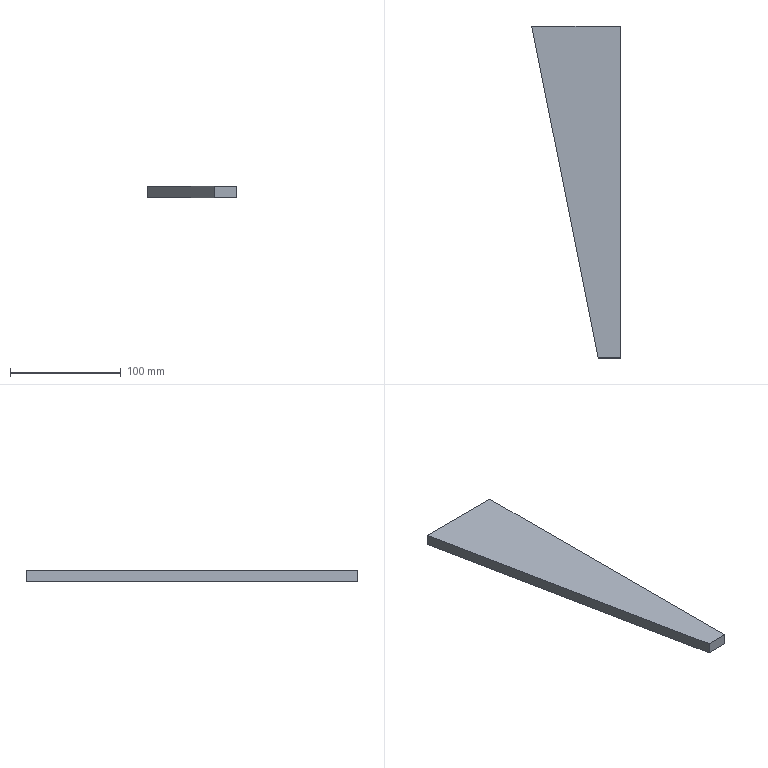Part | SolidWorks | features Extrusion 1 | 1 solid | 6 faces | box 80 x 300 x 10 mm | volume 150000 mm3 | plane 6
STEP:
#1=CARTESIAN_POINT('',(-80.,0.,-5.));
#2=VERTEX_POINT('',#1);
#3=CARTESIAN_POINT('',(-20.,-300.,-5.));
#4=VERTEX_POINT('',#3);
#5=CARTESIAN_POINT('',(-20.,-300.,-5.));
#6=DIRECTION('',(0.1961,-0.9806,0.));
#7=VECTOR('',#6,1000.);
#8=LINE('',#5,#7);
#9=EDGE_CURVE('',#2,#4,#8,.T.);
#10=ORIENTED_EDGE('',*,*,#9,.T.);
#11=CARTESIAN_POINT('',(-20.,-300.,5.));
#12=VERTEX_POINT('',#11);
#13=CARTESIAN_POINT('',(-20.,-300.,5.));
#14=DIRECTION('',(0.,0.,-1.));
#15=VECTOR('',#14,1000.);
#16=LINE('',#13,#15);
#17=EDGE_CURVE('',#12,#4,#16,.T.);
#18=ORIENTED_EDGE('',*,*,#17,.F.);
#19=CARTESIAN_POINT('',(-80.,0.,5.));
#20=VERTEX_POINT('',#19);
#21=CARTESIAN_POINT('',(-20.,-300.,5.));
#22=DIRECTION('',(0.1961,-0.9806,0.));
#23=VECTOR('',#22,1000.);
#24=LINE('',#21,#23);
#25=EDGE_CURVE('',#20,#12,#24,.T.);
#26=ORIENTED_EDGE('',*,*,#25,.F.);
#27=CARTESIAN_POINT('',(-80.,0.,5.));
#28=DIRECTION('',(0.,0.,-1.));
#29=VECTOR('',#28,1000.);
#30=LINE('',#27,#29);
#31=EDGE_CURVE('',#20,#2,#30,.T.);
#32=ORIENTED_EDGE('',*,*,#31,.T.);
#33=EDGE_LOOP('',(#10,#18,#26,#32));
#34=FACE_OUTER_BOUND('',#33,.T.);
#35=CARTESIAN_POINT('',(-20.,-300.,5.));
#36=DIRECTION('',(0.9806,0.1961,0.));
#37=DIRECTION('',(-0.1961,0.9806,0.));
#38=AXIS2_PLACEMENT_3D('',#35,#36,#37);
#39=PLANE('',#38);
#40=ADVANCED_FACE('',(#34),#39,.F.);
#41=CARTESIAN_POINT('',(0.,-300.,-5.));
#42=VERTEX_POINT('',#41);
#43=CARTESIAN_POINT('',(0.,-300.,-5.));
#44=DIRECTION('',(1.,0.,0.));
#45=VECTOR('',#44,1000.);
#46=LINE('',#43,#45);
#47=EDGE_CURVE('',#4,#42,#46,.T.);
#48=ORIENTED_EDGE('',*,*,#47,.T.);
#49=CARTESIAN_POINT('',(0.,-300.,5.));
#50=VERTEX_POINT('',#49);
#51=CARTESIAN_POINT('',(0.,-300.,5.));
#52=DIRECTION('',(0.,0.,-1.));
#53=VECTOR('',#52,1000.);
#54=LINE('',#51,#53);
#55=EDGE_CURVE('',#50,#42,#54,.T.);
#56=ORIENTED_EDGE('',*,*,#55,.F.);
#57=CARTESIAN_POINT('',(0.,-300.,5.));
#58=DIRECTION('',(1.,0.,0.));
#59=VECTOR('',#58,1000.);
#60=LINE('',#57,#59);
#61=EDGE_CURVE('',#12,#50,#60,.T.);
#62=ORIENTED_EDGE('',*,*,#61,.F.);
#63=ORIENTED_EDGE('',*,*,#17,.T.);
#64=EDGE_LOOP('',(#48,#56,#62,#63));
#65=FACE_OUTER_BOUND('',#64,.T.);
#66=CARTESIAN_POINT('',(0.,-300.,5.));
#67=DIRECTION('',(0.,1.,0.));
#68=DIRECTION('',(0.,0.,1.));
#69=AXIS2_PLACEMENT_3D('',#66,#67,#68);
#70=PLANE('',#69);
#71=ADVANCED_FACE('',(#65),#70,.F.);
#72=CARTESIAN_POINT('',(0.,0.,-5.));
#73=VERTEX_POINT('',#72);
#74=CARTESIAN_POINT('',(0.,0.,-5.));
#75=DIRECTION('',(0.,1.,0.));
#76=VECTOR('',#75,1000.);
#77=LINE('',#74,#76);
#78=EDGE_CURVE('',#42,#73,#77,.T.);
#79=ORIENTED_EDGE('',*,*,#78,.T.);
#80=CARTESIAN_POINT('',(0.,0.,5.));
#81=VERTEX_POINT('',#80);
#82=CARTESIAN_POINT('',(0.,0.,5.));
#83=DIRECTION('',(0.,0.,-1.));
#84=VECTOR('',#83,1000.);
#85=LINE('',#82,#84);
#86=EDGE_CURVE('',#81,#73,#85,.T.);
#87=ORIENTED_EDGE('',*,*,#86,.F.);
#88=CARTESIAN_POINT('',(0.,0.,5.));
#89=DIRECTION('',(0.,1.,0.));
#90=VECTOR('',#89,1000.);
#91=LINE('',#88,#90);
#92=EDGE_CURVE('',#50,#81,#91,.T.);
#93=ORIENTED_EDGE('',*,*,#92,.F.);
#94=ORIENTED_EDGE('',*,*,#55,.T.);
#95=EDGE_LOOP('',(#79,#87,#93,#94));
#96=FACE_OUTER_BOUND('',#95,.T.);
#97=CARTESIAN_POINT('',(0.,0.,5.));
#98=DIRECTION('',(-1.,0.,0.));
#99=DIRECTION('',(0.,-1.,0.));
#100=AXIS2_PLACEMENT_3D('',#97,#98,#99);
#101=PLANE('',#100);
#102=ADVANCED_FACE('',(#96),#101,.F.);
#103=CARTESIAN_POINT('',(-80.,0.,-5.));
#104=DIRECTION('',(-1.,0.,0.));
#105=VECTOR('',#104,1000.);
#106=LINE('',#103,#105);
#107=EDGE_CURVE('',#73,#2,#106,.T.);
#108=ORIENTED_EDGE('',*,*,#107,.T.);
#109=ORIENTED_EDGE('',*,*,#31,.F.);
#110=CARTESIAN_POINT('',(-80.,0.,5.));
#111=DIRECTION('',(-1.,0.,0.));
#112=VECTOR('',#111,1000.);
#113=LINE('',#110,#112);
#114=EDGE_CURVE('',#81,#20,#113,.T.);
#115=ORIENTED_EDGE('',*,*,#114,.F.);
#116=ORIENTED_EDGE('',*,*,#86,.T.);
#117=EDGE_LOOP('',(#108,#109,#115,#116));
#118=FACE_OUTER_BOUND('',#117,.T.);
#119=CARTESIAN_POINT('',(-80.,0.,5.));
#120=DIRECTION('',(0.,-1.,0.));
#121=DIRECTION('',(0.,0.,-1.));
#122=AXIS2_PLACEMENT_3D('',#119,#120,#121);
#123=PLANE('',#122);
#124=ADVANCED_FACE('',(#118),#123,.F.);
#125=ORIENTED_EDGE('',*,*,#25,.T.);
#126=ORIENTED_EDGE('',*,*,#61,.T.);
#127=ORIENTED_EDGE('',*,*,#92,.T.);
#128=ORIENTED_EDGE('',*,*,#114,.T.);
#129=EDGE_LOOP('',(#125,#126,#127,#128));
#130=FACE_OUTER_BOUND('',#129,.T.);
#131=CARTESIAN_POINT('',(-80.,0.,5.));
#132=DIRECTION('',(0.,0.,-1.));
#133=DIRECTION('',(-1.,0.,0.));
#134=AXIS2_PLACEMENT_3D('',#131,#132,#133);
#135=PLANE('',#134);
#136=ADVANCED_FACE('',(#130),#135,.F.);
#137=ORIENTED_EDGE('',*,*,#9,.F.);
#138=ORIENTED_EDGE('',*,*,#107,.F.);
#139=ORIENTED_EDGE('',*,*,#78,.F.);
#140=ORIENTED_EDGE('',*,*,#47,.F.);
#141=EDGE_LOOP('',(#137,#138,#139,#140));
#142=FACE_OUTER_BOUND('',#141,.T.);
#143=CARTESIAN_POINT('',(-80.,0.,-5.));
#144=DIRECTION('',(0.,0.,-1.));
#145=DIRECTION('',(-1.,0.,0.));
#146=AXIS2_PLACEMENT_3D('',#143,#144,#145);
#147=PLANE('',#146);
#148=ADVANCED_FACE('',(#142),#147,.T.);
#149=CLOSED_SHELL('',(#40,#71,#102,#124,#136,#148));
#150=MANIFOLD_SOLID_BREP('',#149);
#151=CARTESIAN_POINT('',(0.,0.,0.));
#152=DIRECTION('',(0.,0.,1.));
#153=DIRECTION('',(1.,0.,0.));
#154=AXIS2_PLACEMENT_3D('',#151,#152,#153);
#155=(LENGTH_UNIT()NAMED_UNIT(*)SI_UNIT(.MILLI.,.METRE.));
#156=UNCERTAINTY_MEASURE_WITH_UNIT(LENGTH_MEASURE(0.00001),#155,'','');
#157=(NAMED_UNIT(*)PLANE_ANGLE_UNIT()SI_UNIT($,.RADIAN.));
#158=(NAMED_UNIT(*)SI_UNIT($,.STERADIAN.)SOLID_ANGLE_UNIT());
#159=(GEOMETRIC_REPRESENTATION_CONTEXT(3)GLOBAL_UNCERTAINTY_ASSIGNED_CONTEXT((#156))GLOBAL_UNIT_ASSIGNED_CONTEXT((#155,#157,#158))REPRESENTATION_CONTEXT('',''));
#160=ADVANCED_BREP_SHAPE_REPRESENTATION('',(#150,#154),#159);